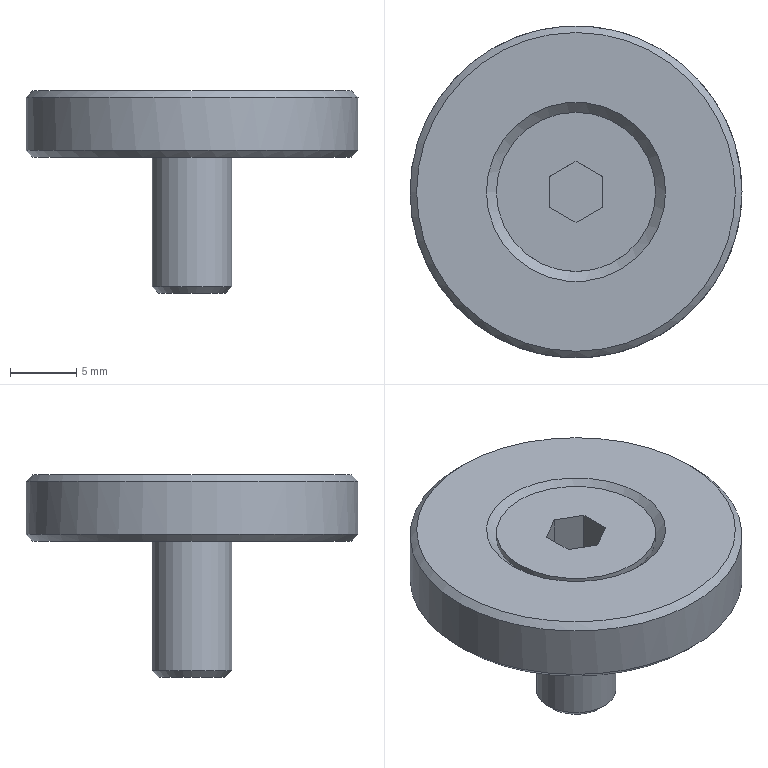Part | STEP file | LJD | 2 solids | 20 faces | box 25 x 25 x 15.25 mm | volume 2621 mm3 | plane 11 | cone 5 | cylinder 4 | commonest cylinder face diameters 6 x1 6.5 x1 12 x1 25 x1